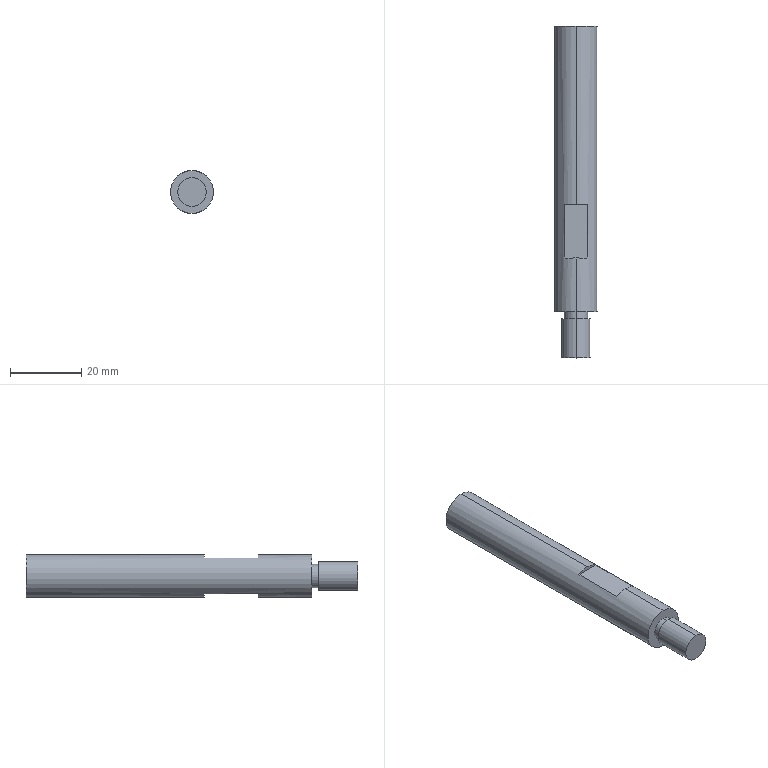Part | STEP file | PN_0059 pillar | 1 solid | 20 faces | box 12 x 93 x 12 mm | volume 9356 mm3 | plane 10 | cylinder 8 | cone 2 | commonest cylinder face diameters 4.2 x2 6.6 x2 8 x2 12 x2
STEP:
#1=CARTESIAN_POINT('',(0.,0.,0.));
#2=DIRECTION('',(0.,0.,1.));
#3=DIRECTION('',(1.,0.,0.));
#4=AXIS2_PLACEMENT_3D('',#1,#2,#3);
#5=CARTESIAN_POINT('',(0.,11.,-4.));
#6=VERTEX_POINT('',#5);
#7=CARTESIAN_POINT('',(0.,11.,4.));
#8=VERTEX_POINT('',#7);
#9=CARTESIAN_POINT('',(0.,11.,0.));
#10=DIRECTION('',(0.,-1.,0.));
#11=DIRECTION('',(0.,0.,-1.));
#12=AXIS2_PLACEMENT_3D('',#9,#10,#11);
#13=CIRCLE('',#12,4.);
#14=CARTESIAN_POINT('',(0.,0.,0.));
#15=DIRECTION('',(0.,-1.,0.));
#16=DIRECTION('',(0.,0.,-1.));
#17=AXIS2_PLACEMENT_3D('',#14,#15,#16);
#18=CYLINDRICAL_SURFACE('',#17,4.);
#19=CARTESIAN_POINT('',(0.,-11.));
#20=DIRECTION('',(1.,0.));
#21=VECTOR('',#20,1.);
#22=LINE('',#19,#21);
#23=(GEOMETRIC_REPRESENTATION_CONTEXT(2)PARAMETRIC_REPRESENTATION_CONTEXT()REPRESENTATION_CONTEXT('',''));
#24=DEFINITIONAL_REPRESENTATION('',(#22),#23);
#25=PCURVE('',#18,#24);
#26=CARTESIAN_POINT('',(4.,11.,0.));
#27=DIRECTION('',(0.,-1.,0.));
#28=DIRECTION('',(0.,0.,-1.));
#29=AXIS2_PLACEMENT_3D('',#26,#27,#28);
#30=PLANE('',#29);
#31=CARTESIAN_POINT('',(0.,-4.));
#32=DIRECTION('',(1.,0.));
#33=AXIS2_PLACEMENT_2D('',#31,#32);
#34=CIRCLE('',#33,4.);
#35=(GEOMETRIC_REPRESENTATION_CONTEXT(2)PARAMETRIC_REPRESENTATION_CONTEXT()REPRESENTATION_CONTEXT('',''));
#36=DEFINITIONAL_REPRESENTATION('',(#34),#35);
#37=PCURVE('',#30,#36);
#38=SURFACE_CURVE('',#13,(#25,#37),.PCURVE_S1.);
#39=EDGE_CURVE('',#6,#8,#38,.T.);
#40=ORIENTED_EDGE('',*,*,#39,.T.);
#41=CARTESIAN_POINT('',(0.,0.,4.));
#42=VERTEX_POINT('',#41);
#43=CARTESIAN_POINT('',(0.,0.,4.));
#44=DIRECTION('',(0.,-1.,0.));
#45=VECTOR('',#44,1.);
#46=LINE('',#43,#45);
#47=CARTESIAN_POINT('',(3.142,0.));
#48=DIRECTION('',(0.,1.));
#49=VECTOR('',#48,1.);
#50=LINE('',#47,#49);
#51=(GEOMETRIC_REPRESENTATION_CONTEXT(2)PARAMETRIC_REPRESENTATION_CONTEXT()REPRESENTATION_CONTEXT('',''));
#52=DEFINITIONAL_REPRESENTATION('',(#50),#51);
#53=PCURVE('',#18,#52);
#54=CARTESIAN_POINT('',(0.,0.,0.));
#55=DIRECTION('',(0.,-1.,0.));
#56=DIRECTION('',(0.,0.,-1.));
#57=AXIS2_PLACEMENT_3D('',#54,#55,#56);
#58=CYLINDRICAL_SURFACE('',#57,4.);
#59=CARTESIAN_POINT('',(3.142,0.));
#60=DIRECTION('',(0.,1.));
#61=VECTOR('',#60,1.);
#62=LINE('',#59,#61);
#63=(GEOMETRIC_REPRESENTATION_CONTEXT(2)PARAMETRIC_REPRESENTATION_CONTEXT()REPRESENTATION_CONTEXT('',''));
#64=DEFINITIONAL_REPRESENTATION('',(#62),#63);
#65=PCURVE('',#58,#64);
#66=SURFACE_CURVE('',#46,(#53,#65),.PCURVE_S1.);
#67=EDGE_CURVE('',#8,#42,#66,.T.);
#68=ORIENTED_EDGE('',*,*,#67,.T.);
#69=CARTESIAN_POINT('',(0.,0.,-4.));
#70=VERTEX_POINT('',#69);
#71=CARTESIAN_POINT('',(0.,0.,0.));
#72=DIRECTION('',(0.,-1.,0.));
#73=DIRECTION('',(0.,0.,-1.));
#74=AXIS2_PLACEMENT_3D('',#71,#72,#73);
#75=CIRCLE('',#74,4.);
#76=CARTESIAN_POINT('',(0.,0.));
#77=DIRECTION('',(1.,0.));
#78=VECTOR('',#77,1.);
#79=LINE('',#76,#78);
#80=(GEOMETRIC_REPRESENTATION_CONTEXT(2)PARAMETRIC_REPRESENTATION_CONTEXT()REPRESENTATION_CONTEXT('',''));
#81=DEFINITIONAL_REPRESENTATION('',(#79),#80);
#82=PCURVE('',#18,#81);
#83=CARTESIAN_POINT('',(0.,0.,0.));
#84=DIRECTION('',(0.,-1.,0.));
#85=DIRECTION('',(0.,0.,-1.));
#86=AXIS2_PLACEMENT_3D('',#83,#84,#85);
#87=PLANE('',#86);
#88=CARTESIAN_POINT('',(0.,0.));
#89=DIRECTION('',(1.,0.));
#90=AXIS2_PLACEMENT_2D('',#88,#89);
#91=CIRCLE('',#90,4.);
#92=(GEOMETRIC_REPRESENTATION_CONTEXT(2)PARAMETRIC_REPRESENTATION_CONTEXT()REPRESENTATION_CONTEXT('',''));
#93=DEFINITIONAL_REPRESENTATION('',(#91),#92);
#94=PCURVE('',#87,#93);
#95=SURFACE_CURVE('',#75,(#82,#94),.PCURVE_S1.);
#96=EDGE_CURVE('',#70,#42,#95,.T.);
#97=ORIENTED_EDGE('',*,*,#96,.F.);
#98=CARTESIAN_POINT('',(0.,0.,-4.));
#99=DIRECTION('',(0.,-1.,0.));
#100=VECTOR('',#99,1.);
#101=LINE('',#98,#100);
#102=CARTESIAN_POINT('',(0.,0.));
#103=DIRECTION('',(0.,1.));
#104=VECTOR('',#103,1.);
#105=LINE('',#102,#104);
#106=(GEOMETRIC_REPRESENTATION_CONTEXT(2)PARAMETRIC_REPRESENTATION_CONTEXT()REPRESENTATION_CONTEXT('',''));
#107=DEFINITIONAL_REPRESENTATION('',(#105),#106);
#108=PCURVE('',#18,#107);
#109=CARTESIAN_POINT('',(6.283,0.));
#110=DIRECTION('',(0.,1.));
#111=VECTOR('',#110,1.);
#112=LINE('',#109,#111);
#113=(GEOMETRIC_REPRESENTATION_CONTEXT(2)PARAMETRIC_REPRESENTATION_CONTEXT()REPRESENTATION_CONTEXT('',''));
#114=DEFINITIONAL_REPRESENTATION('',(#112),#113);
#115=PCURVE('',#58,#114);
#116=SURFACE_CURVE('',#101,(#108,#115),.PCURVE_S1.);
#117=EDGE_CURVE('',#6,#70,#116,.T.);
#118=ORIENTED_EDGE('',*,*,#117,.F.);
#119=EDGE_LOOP('',(#40,#68,#97,#118));
#120=FACE_BOUND('',#119,.T.);
#121=ADVANCED_FACE('',(#120),#18,.T.);
#122=CARTESIAN_POINT('',(0.,13.,-3.3));
#123=VERTEX_POINT('',#122);
#124=CARTESIAN_POINT('',(0.,13.,3.3));
#125=VERTEX_POINT('',#124);
#126=CARTESIAN_POINT('',(0.,13.,0.));
#127=DIRECTION('',(0.,-1.,0.));
#128=DIRECTION('',(0.,0.,-1.));
#129=AXIS2_PLACEMENT_3D('',#126,#127,#128);
#130=CIRCLE('',#129,3.3);
#131=CARTESIAN_POINT('',(0.,0.,0.));
#132=DIRECTION('',(0.,-1.,0.));
#133=DIRECTION('',(0.,0.,-1.));
#134=AXIS2_PLACEMENT_3D('',#131,#132,#133);
#135=CYLINDRICAL_SURFACE('',#134,3.3);
#136=CARTESIAN_POINT('',(0.,-13.));
#137=DIRECTION('',(1.,0.));
#138=VECTOR('',#137,1.);
#139=LINE('',#136,#138);
#140=(GEOMETRIC_REPRESENTATION_CONTEXT(2)PARAMETRIC_REPRESENTATION_CONTEXT()REPRESENTATION_CONTEXT('',''));
#141=DEFINITIONAL_REPRESENTATION('',(#139),#140);
#142=PCURVE('',#135,#141);
#143=CARTESIAN_POINT('',(4.,13.,0.));
#144=DIRECTION('',(0.,-1.,0.));
#145=DIRECTION('',(0.,0.,-1.));
#146=AXIS2_PLACEMENT_3D('',#143,#144,#145);
#147=PLANE('',#146);
#148=CARTESIAN_POINT('',(0.,-4.));
#149=DIRECTION('',(1.,0.));
#150=AXIS2_PLACEMENT_2D('',#148,#149);
#151=CIRCLE('',#150,3.3);
#152=(GEOMETRIC_REPRESENTATION_CONTEXT(2)PARAMETRIC_REPRESENTATION_CONTEXT()REPRESENTATION_CONTEXT('',''));
#153=DEFINITIONAL_REPRESENTATION('',(#151),#152);
#154=PCURVE('',#147,#153);
#155=SURFACE_CURVE('',#130,(#142,#154),.PCURVE_S1.);
#156=EDGE_CURVE('',#123,#125,#155,.T.);
#157=ORIENTED_EDGE('',*,*,#156,.T.);
#158=CARTESIAN_POINT('',(0.,11.,3.3));
#159=VERTEX_POINT('',#158);
#160=CARTESIAN_POINT('',(0.,0.,3.3));
#161=DIRECTION('',(0.,-1.,0.));
#162=VECTOR('',#161,1.);
#163=LINE('',#160,#162);
#164=CARTESIAN_POINT('',(3.142,0.));
#165=DIRECTION('',(0.,1.));
#166=VECTOR('',#165,1.);
#167=LINE('',#164,#166);
#168=(GEOMETRIC_REPRESENTATION_CONTEXT(2)PARAMETRIC_REPRESENTATION_CONTEXT()REPRESENTATION_CONTEXT('',''));
#169=DEFINITIONAL_REPRESENTATION('',(#167),#168);
#170=PCURVE('',#135,#169);
#171=CARTESIAN_POINT('',(0.,0.,0.));
#172=DIRECTION('',(0.,-1.,0.));
#173=DIRECTION('',(0.,0.,-1.));
#174=AXIS2_PLACEMENT_3D('',#171,#172,#173);
#175=CYLINDRICAL_SURFACE('',#174,3.3);
#176=CARTESIAN_POINT('',(3.142,0.));
#177=DIRECTION('',(0.,1.));
#178=VECTOR('',#177,1.);
#179=LINE('',#176,#178);
#180=(GEOMETRIC_REPRESENTATION_CONTEXT(2)PARAMETRIC_REPRESENTATION_CONTEXT()REPRESENTATION_CONTEXT('',''));
#181=DEFINITIONAL_REPRESENTATION('',(#179),#180);
#182=PCURVE('',#175,#181);
#183=SURFACE_CURVE('',#163,(#170,#182),.PCURVE_S1.);
#184=EDGE_CURVE('',#125,#159,#183,.T.);
#185=ORIENTED_EDGE('',*,*,#184,.T.);
#186=CARTESIAN_POINT('',(0.,11.,-3.3));
#187=VERTEX_POINT('',#186);
#188=CARTESIAN_POINT('',(0.,11.,0.));
#189=DIRECTION('',(0.,-1.,0.));
#190=DIRECTION('',(0.,0.,-1.));
#191=AXIS2_PLACEMENT_3D('',#188,#189,#190);
#192=CIRCLE('',#191,3.3);
#193=CARTESIAN_POINT('',(0.,-11.));
#194=DIRECTION('',(1.,0.));
#195=VECTOR('',#194,1.);
#196=LINE('',#193,#195);
#197=(GEOMETRIC_REPRESENTATION_CONTEXT(2)PARAMETRIC_REPRESENTATION_CONTEXT()REPRESENTATION_CONTEXT('',''));
#198=DEFINITIONAL_REPRESENTATION('',(#196),#197);
#199=PCURVE('',#135,#198);
#200=CARTESIAN_POINT('',(0.,-4.));
#201=DIRECTION('',(1.,0.));
#202=AXIS2_PLACEMENT_2D('',#200,#201);
#203=CIRCLE('',#202,3.3);
#204=(GEOMETRIC_REPRESENTATION_CONTEXT(2)PARAMETRIC_REPRESENTATION_CONTEXT()REPRESENTATION_CONTEXT('',''));
#205=DEFINITIONAL_REPRESENTATION('',(#203),#204);
#206=PCURVE('',#30,#205);
#207=SURFACE_CURVE('',#192,(#199,#206),.PCURVE_S1.);
#208=EDGE_CURVE('',#187,#159,#207,.T.);
#209=ORIENTED_EDGE('',*,*,#208,.F.);
#210=CARTESIAN_POINT('',(0.,0.,-3.3));
#211=DIRECTION('',(0.,-1.,0.));
#212=VECTOR('',#211,1.);
#213=LINE('',#210,#212);
#214=CARTESIAN_POINT('',(0.,0.));
#215=DIRECTION('',(0.,1.));
#216=VECTOR('',#215,1.);
#217=LINE('',#214,#216);
#218=(GEOMETRIC_REPRESENTATION_CONTEXT(2)PARAMETRIC_REPRESENTATION_CONTEXT()REPRESENTATION_CONTEXT('',''));
#219=DEFINITIONAL_REPRESENTATION('',(#217),#218);
#220=PCURVE('',#135,#219);
#221=CARTESIAN_POINT('',(6.283,0.));
#222=DIRECTION('',(0.,1.));
#223=VECTOR('',#222,1.);
#224=LINE('',#221,#223);
#225=(GEOMETRIC_REPRESENTATION_CONTEXT(2)PARAMETRIC_REPRESENTATION_CONTEXT()REPRESENTATION_CONTEXT('',''));
#226=DEFINITIONAL_REPRESENTATION('',(#224),#225);
#227=PCURVE('',#175,#226);
#228=SURFACE_CURVE('',#213,(#220,#227),.PCURVE_S1.);
#229=EDGE_CURVE('',#123,#187,#228,.T.);
#230=ORIENTED_EDGE('',*,*,#229,.F.);
#231=EDGE_LOOP('',(#157,#185,#209,#230));
#232=FACE_BOUND('',#231,.T.);
#233=ADVANCED_FACE('',(#232),#135,.T.);
#234=CARTESIAN_POINT('',(0.,80.6,2.1));
#235=VERTEX_POINT('',#234);
#236=CARTESIAN_POINT('',(0.,93.,2.1));
#237=VERTEX_POINT('',#236);
#238=CARTESIAN_POINT('',(0.,93.,2.1));
#239=DIRECTION('',(0.,1.,0.));
#240=VECTOR('',#239,1.);
#241=LINE('',#238,#240);
#242=CARTESIAN_POINT('',(0.,93.,0.));
#243=DIRECTION('',(0.,1.,0.));
#244=DIRECTION('',(0.,0.,1.));
#245=AXIS2_PLACEMENT_3D('',#242,#243,#244);
#246=CYLINDRICAL_SURFACE('',#245,2.1);
#247=CARTESIAN_POINT('',(6.283,0.));
#248=DIRECTION('',(0.,1.));
#249=VECTOR('',#248,1.);
#250=LINE('',#247,#249);
#251=(GEOMETRIC_REPRESENTATION_CONTEXT(2)PARAMETRIC_REPRESENTATION_CONTEXT()REPRESENTATION_CONTEXT('',''));
#252=DEFINITIONAL_REPRESENTATION('',(#250),#251);
#253=PCURVE('',#246,#252);
#254=CARTESIAN_POINT('',(0.,93.,0.));
#255=DIRECTION('',(0.,1.,0.));
#256=DIRECTION('',(0.,0.,1.));
#257=AXIS2_PLACEMENT_3D('',#254,#255,#256);
#258=CYLINDRICAL_SURFACE('',#257,2.1);
#259=CARTESIAN_POINT('',(0.,0.));
#260=DIRECTION('',(0.,1.));
#261=VECTOR('',#260,1.);
#262=LINE('',#259,#261);
#263=(GEOMETRIC_REPRESENTATION_CONTEXT(2)PARAMETRIC_REPRESENTATION_CONTEXT()REPRESENTATION_CONTEXT('',''));
#264=DEFINITIONAL_REPRESENTATION('',(#262),#263);
#265=PCURVE('',#258,#264);
#266=SURFACE_CURVE('',#241,(#253,#265),.PCURVE_S1.);
#267=EDGE_CURVE('',#235,#237,#266,.T.);
#268=ORIENTED_EDGE('',*,*,#267,.T.);
#269=CARTESIAN_POINT('',(0.,93.,-2.1));
#270=VERTEX_POINT('',#269);
#271=CARTESIAN_POINT('',(0.,93.,0.));
#272=DIRECTION('',(0.,1.,0.));
#273=DIRECTION('',(0.,0.,1.));
#274=AXIS2_PLACEMENT_3D('',#271,#272,#273);
#275=CIRCLE('',#274,2.1);
#276=CARTESIAN_POINT('',(0.,0.));
#277=DIRECTION('',(1.,0.));
#278=VECTOR('',#277,1.);
#279=LINE('',#276,#278);
#280=(GEOMETRIC_REPRESENTATION_CONTEXT(2)PARAMETRIC_REPRESENTATION_CONTEXT()REPRESENTATION_CONTEXT('',''));
#281=DEFINITIONAL_REPRESENTATION('',(#279),#280);
#282=PCURVE('',#246,#281);
#283=CARTESIAN_POINT('',(6.,93.,0.));
#284=DIRECTION('',(0.,1.,0.));
#285=DIRECTION('',(0.,0.,1.));
#286=AXIS2_PLACEMENT_3D('',#283,#284,#285);
#287=PLANE('',#286);
#288=CARTESIAN_POINT('',(0.,-6.));
#289=DIRECTION('',(1.,0.));
#290=AXIS2_PLACEMENT_2D('',#288,#289);
#291=CIRCLE('',#290,2.1);
#292=(GEOMETRIC_REPRESENTATION_CONTEXT(2)PARAMETRIC_REPRESENTATION_CONTEXT()REPRESENTATION_CONTEXT('',''));
#293=DEFINITIONAL_REPRESENTATION('',(#291),#292);
#294=PCURVE('',#287,#293);
#295=SURFACE_CURVE('',#275,(#282,#294),.PCURVE_S1.);
#296=EDGE_CURVE('',#270,#237,#295,.T.);
#297=ORIENTED_EDGE('',*,*,#296,.F.);
#298=CARTESIAN_POINT('',(0.,80.6,-2.1));
#299=VERTEX_POINT('',#298);
#300=CARTESIAN_POINT('',(0.,93.,-2.1));
#301=DIRECTION('',(0.,1.,0.));
#302=VECTOR('',#301,1.);
#303=LINE('',#300,#302);
#304=CARTESIAN_POINT('',(3.142,0.));
#305=DIRECTION('',(0.,1.));
#306=VECTOR('',#305,1.);
#307=LINE('',#304,#306);
#308=(GEOMETRIC_REPRESENTATION_CONTEXT(2)PARAMETRIC_REPRESENTATION_CONTEXT()REPRESENTATION_CONTEXT('',''));
#309=DEFINITIONAL_REPRESENTATION('',(#307),#308);
#310=PCURVE('',#246,#309);
#311=CARTESIAN_POINT('',(3.142,0.));
#312=DIRECTION('',(0.,1.));
#313=VECTOR('',#312,1.);
#314=LINE('',#311,#313);
#315=(GEOMETRIC_REPRESENTATION_CONTEXT(2)PARAMETRIC_REPRESENTATION_CONTEXT()REPRESENTATION_CONTEXT('',''));
#316=DEFINITIONAL_REPRESENTATION('',(#314),#315);
#317=PCURVE('',#258,#316);
#318=SURFACE_CURVE('',#303,(#310,#317),.PCURVE_S1.);
#319=EDGE_CURVE('',#299,#270,#318,.T.);
#320=ORIENTED_EDGE('',*,*,#319,.F.);
#321=CARTESIAN_POINT('',(0.,80.6,0.));
#322=DIRECTION('',(0.,1.,0.));
#323=DIRECTION('',(0.,0.,1.));
#324=AXIS2_PLACEMENT_3D('',#321,#322,#323);
#325=CIRCLE('',#324,2.1);
#326=CARTESIAN_POINT('',(0.,-12.4));
#327=DIRECTION('',(1.,0.));
#328=VECTOR('',#327,1.);
#329=LINE('',#326,#328);
#330=(GEOMETRIC_REPRESENTATION_CONTEXT(2)PARAMETRIC_REPRESENTATION_CONTEXT()REPRESENTATION_CONTEXT('',''));
#331=DEFINITIONAL_REPRESENTATION('',(#329),#330);
#332=PCURVE('',#246,#331);
#333=CARTESIAN_POINT('',(0.,80.6,0.));
#334=DIRECTION('',(0.,1.,0.));
#335=DIRECTION('',(0.,0.,1.));
#336=AXIS2_PLACEMENT_3D('',#333,#334,#335);
#337=CONICAL_SURFACE('',#336,2.1,1.03);
#338=CARTESIAN_POINT('',(0.,0.));
#339=DIRECTION('',(1.,0.));
#340=VECTOR('',#339,1.);
#341=LINE('',#338,#340);
#342=(GEOMETRIC_REPRESENTATION_CONTEXT(2)PARAMETRIC_REPRESENTATION_CONTEXT()REPRESENTATION_CONTEXT('',''));
#343=DEFINITIONAL_REPRESENTATION('',(#341),#342);
#344=PCURVE('',#337,#343);
#345=SURFACE_CURVE('',#325,(#332,#344),.PCURVE_S1.);
#346=EDGE_CURVE('',#299,#235,#345,.T.);
#347=ORIENTED_EDGE('',*,*,#346,.T.);
#348=EDGE_LOOP('',(#268,#297,#320,#347));
#349=FACE_BOUND('',#348,.F.);
#350=ADVANCED_FACE('',(#349),#246,.F.);
#351=ORIENTED_EDGE('',*,*,#346,.F.);
#352=CARTESIAN_POINT('',(0.,79.338,0.));
#353=VERTEX_POINT('',#352);
#354=CARTESIAN_POINT('',(0.,80.6,-2.1));
#355=DIRECTION('',(0.,0.515,-0.8572));
#356=VECTOR('',#355,1.);
#357=LINE('',#354,#356);
#358=CARTESIAN_POINT('',(3.142,0.));
#359=DIRECTION('',(0.,1.));
#360=VECTOR('',#359,1.);
#361=LINE('',#358,#360);
#362=(GEOMETRIC_REPRESENTATION_CONTEXT(2)PARAMETRIC_REPRESENTATION_CONTEXT()REPRESENTATION_CONTEXT('',''));
#363=DEFINITIONAL_REPRESENTATION('',(#361),#362);
#364=PCURVE('',#337,#363);
#365=CARTESIAN_POINT('',(0.,80.6,0.));
#366=DIRECTION('',(0.,1.,0.));
#367=DIRECTION('',(0.,0.,1.));
#368=AXIS2_PLACEMENT_3D('',#365,#366,#367);
#369=CONICAL_SURFACE('',#368,2.1,1.03);
#370=CARTESIAN_POINT('',(3.142,0.));
#371=DIRECTION('',(0.,1.));
#372=VECTOR('',#371,1.);
#373=LINE('',#370,#372);
#374=(GEOMETRIC_REPRESENTATION_CONTEXT(2)PARAMETRIC_REPRESENTATION_CONTEXT()REPRESENTATION_CONTEXT('',''));
#375=DEFINITIONAL_REPRESENTATION('',(#373),#374);
#376=PCURVE('',#369,#375);
#377=SURFACE_CURVE('',#357,(#364,#376),.PCURVE_S1.);
#378=EDGE_CURVE('',#353,#299,#377,.T.);
#379=ORIENTED_EDGE('',*,*,#378,.F.);
#380=CARTESIAN_POINT('',(0.,80.6,2.1));
#381=DIRECTION('',(0.,0.515,0.8572));
#382=VECTOR('',#381,1.);
#383=LINE('',#380,#382);
#384=CARTESIAN_POINT('',(6.283,0.));
#385=DIRECTION('',(0.,1.));
#386=VECTOR('',#385,1.);
#387=LINE('',#384,#386);
#388=(GEOMETRIC_REPRESENTATION_CONTEXT(2)PARAMETRIC_REPRESENTATION_CONTEXT()REPRESENTATION_CONTEXT('',''));
#389=DEFINITIONAL_REPRESENTATION('',(#387),#388);
#390=PCURVE('',#337,#389);
#391=CARTESIAN_POINT('',(0.,0.));
#392=DIRECTION('',(0.,1.));
#393=VECTOR('',#392,1.);
#394=LINE('',#391,#393);
#395=(GEOMETRIC_REPRESENTATION_CONTEXT(2)PARAMETRIC_REPRESENTATION_CONTEXT()REPRESENTATION_CONTEXT('',''));
#396=DEFINITIONAL_REPRESENTATION('',(#394),#395);
#397=PCURVE('',#369,#396);
#398=SURFACE_CURVE('',#383,(#390,#397),.PCURVE_S1.);
#399=EDGE_CURVE('',#353,#235,#398,.T.);
#400=ORIENTED_EDGE('',*,*,#399,.T.);
#401=EDGE_LOOP('',(#351,#379,#400));
#402=FACE_BOUND('',#401,.F.);
#403=ADVANCED_FACE('',(#402),#337,.F.);
#404=CARTESIAN_POINT('',(0.,93.,-6.));
#405=VERTEX_POINT('',#404);
#406=CARTESIAN_POINT('',(0.,93.,6.));
#407=VERTEX_POINT('',#406);
#408=CARTESIAN_POINT('',(0.,93.,0.));
#409=DIRECTION('',(0.,-1.,0.));
#410=DIRECTION('',(0.,0.,-1.));
#411=AXIS2_PLACEMENT_3D('',#408,#409,#410);
#412=CIRCLE('',#411,6.);
#413=CARTESIAN_POINT('',(0.,0.,0.));
#414=DIRECTION('',(0.,-1.,0.));
#415=DIRECTION('',(0.,0.,-1.));
#416=AXIS2_PLACEMENT_3D('',#413,#414,#415);
#417=CYLINDRICAL_SURFACE('',#416,6.);
#418=CARTESIAN_POINT('',(0.,-93.));
#419=DIRECTION('',(1.,0.));
#420=VECTOR('',#419,1.);
#421=LINE('',#418,#420);
#422=(GEOMETRIC_REPRESENTATION_CONTEXT(2)PARAMETRIC_REPRESENTATION_CONTEXT()REPRESENTATION_CONTEXT('',''));
#423=DEFINITIONAL_REPRESENTATION('',(#421),#422);
#424=PCURVE('',#417,#423);
#425=CARTESIAN_POINT('',(-6.,-6.));
#426=CARTESIAN_POINT('',(-6.,4.392));
#427=CARTESIAN_POINT('',(3.,-0.8038));
#428=CARTESIAN_POINT('',(12.,-6.));
#429=CARTESIAN_POINT('',(3.,-11.196));
#430=CARTESIAN_POINT('',(-6.,-16.392));
#431=CARTESIAN_POINT('',(-6.,-6.));
#432=(BOUNDED_CURVE()B_SPLINE_CURVE(2,(#425,#426,#427,#428,#429,#430,#431),.UNSPECIFIED.,.T.,.F.)B_SPLINE_CURVE_WITH_KNOTS((1,2,2,2,2,1),(-2.094,0.,2.094,4.189,6.283,8.378),.UNSPECIFIED.)CURVE()GEOMETRIC_REPRESENTATION_ITEM()RATIONAL_B_SPLINE_CURVE((1.,0.5,1.,0.5,1.,0.5,1.))REPRESENTATION_ITEM(''));
#433=(GEOMETRIC_REPRESENTATION_CONTEXT(2)PARAMETRIC_REPRESENTATION_CONTEXT()REPRESENTATION_CONTEXT('',''));
#434=DEFINITIONAL_REPRESENTATION('',(#432),#433);
#435=PCURVE('',#287,#434);
#436=SURFACE_CURVE('',#412,(#424,#435),.PCURVE_S1.);
#437=EDGE_CURVE('',#405,#407,#436,.T.);
#438=ORIENTED_EDGE('',*,*,#437,.T.);
#439=CARTESIAN_POINT('',(0.,43.,6.));
#440=VERTEX_POINT('',#439);
#441=CARTESIAN_POINT('',(0.,0.,6.));
#442=DIRECTION('',(0.,-1.,0.));
#443=VECTOR('',#442,1.);
#444=LINE('',#441,#443);
#445=CARTESIAN_POINT('',(3.142,0.));
#446=DIRECTION('',(0.,1.));
#447=VECTOR('',#446,1.);
#448=LINE('',#445,#447);
#449=(GEOMETRIC_REPRESENTATION_CONTEXT(2)PARAMETRIC_REPRESENTATION_CONTEXT()REPRESENTATION_CONTEXT('',''));
#450=DEFINITIONAL_REPRESENTATION('',(#448),#449);
#451=PCURVE('',#417,#450);
#452=CARTESIAN_POINT('',(0.,0.,0.));
#453=DIRECTION('',(0.,-1.,0.));
#454=DIRECTION('',(0.,0.,-1.));
#455=AXIS2_PLACEMENT_3D('',#452,#453,#454);
#456=CYLINDRICAL_SURFACE('',#455,6.);
#457=CARTESIAN_POINT('',(3.142,0.));
#458=DIRECTION('',(0.,1.));
#459=VECTOR('',#458,1.);
#460=LINE('',#457,#459);
#461=(GEOMETRIC_REPRESENTATION_CONTEXT(2)PARAMETRIC_REPRESENTATION_CONTEXT()REPRESENTATION_CONTEXT('',''));
#462=DEFINITIONAL_REPRESENTATION('',(#460),#461);
#463=PCURVE('',#456,#462);
#464=SURFACE_CURVE('',#444,(#451,#463),.PCURVE_S1.);
#465=EDGE_CURVE('',#407,#440,#464,.T.);
#466=ORIENTED_EDGE('',*,*,#465,.T.);
#467=CARTESIAN_POINT('',(3.317,43.,5.));
#468=VERTEX_POINT('',#467);
#469=CARTESIAN_POINT('',(0.,43.,0.));
#470=DIRECTION('',(0.,-1.,0.));
#471=DIRECTION('',(0.,0.,1.));
#472=AXIS2_PLACEMENT_3D('',#469,#470,#471);
#473=CIRCLE('',#472,6.);
#474=CARTESIAN_POINT('',(-3.142,-43.));
#475=DIRECTION('',(1.,0.));
#476=VECTOR('',#475,1.);
#477=LINE('',#474,#476);
#478=(GEOMETRIC_REPRESENTATION_CONTEXT(2)PARAMETRIC_REPRESENTATION_CONTEXT()REPRESENTATION_CONTEXT('',''));
#479=DEFINITIONAL_REPRESENTATION('',(#477),#478);
#480=PCURVE('',#417,#479);
#481=CARTESIAN_POINT('',(-35.,43.,8.217));
#482=DIRECTION('',(0.,1.,0.));
#483=DIRECTION('',(0.,0.,1.));
#484=AXIS2_PLACEMENT_3D('',#481,#482,#483);
#485=PLANE('',#484);
#486=CARTESIAN_POINT('',(-2.217,35.));
#487=CARTESIAN_POINT('',(-2.217,24.608));
#488=CARTESIAN_POINT('',(-11.217,29.804));
#489=CARTESIAN_POINT('',(-20.217,35.));
#490=CARTESIAN_POINT('',(-11.217,40.196));
#491=CARTESIAN_POINT('',(-2.217,45.392));
#492=CARTESIAN_POINT('',(-2.217,35.));
#493=(BOUNDED_CURVE()B_SPLINE_CURVE(2,(#486,#487,#488,#489,#490,#491,#492),.UNSPECIFIED.,.T.,.F.)B_SPLINE_CURVE_WITH_KNOTS((1,2,2,2,2,1),(-2.094,0.,2.094,4.189,6.283,8.378),.UNSPECIFIED.)CURVE()GEOMETRIC_REPRESENTATION_ITEM()RATIONAL_B_SPLINE_CURVE((1.,0.5,1.,0.5,1.,0.5,1.))REPRESENTATION_ITEM(''));
#494=(GEOMETRIC_REPRESENTATION_CONTEXT(2)PARAMETRIC_REPRESENTATION_CONTEXT()REPRESENTATION_CONTEXT('',''));
#495=DEFINITIONAL_REPRESENTATION('',(#493),#494);
#496=PCURVE('',#485,#495);
#497=SURFACE_CURVE('',#473,(#480,#496),.PCURVE_S1.);
#498=EDGE_CURVE('',#468,#440,#497,.T.);
#499=ORIENTED_EDGE('',*,*,#498,.F.);
#500=CARTESIAN_POINT('',(3.317,28.,5.));
#501=VERTEX_POINT('',#500);
#502=CARTESIAN_POINT('',(3.317,0.,5.));
#503=DIRECTION('',(0.,1.,0.));
#504=VECTOR('',#503,1.);
#505=LINE('',#502,#504);
#506=CARTESIAN_POINT('',(2.556,0.));
#507=DIRECTION('',(0.,-1.));
#508=VECTOR('',#507,1.);
#509=LINE('',#506,#508);
#510=(GEOMETRIC_REPRESENTATION_CONTEXT(2)PARAMETRIC_REPRESENTATION_CONTEXT()REPRESENTATION_CONTEXT('',''));
#511=DEFINITIONAL_REPRESENTATION('',(#509),#510);
#512=PCURVE('',#417,#511);
#513=CARTESIAN_POINT('',(-35.,43.,5.));
#514=DIRECTION('',(0.,0.,-1.));
#515=DIRECTION('',(0.,1.,0.));
#516=AXIS2_PLACEMENT_3D('',#513,#514,#515);
#517=PLANE('',#516);
#518=CARTESIAN_POINT('',(-43.,38.317));
#519=DIRECTION('',(1.,0.));
#520=VECTOR('',#519,1.);
#521=LINE('',#518,#520);
#522=(GEOMETRIC_REPRESENTATION_CONTEXT(2)PARAMETRIC_REPRESENTATION_CONTEXT()REPRESENTATION_CONTEXT('',''));
#523=DEFINITIONAL_REPRESENTATION('',(#521),#522);
#524=PCURVE('',#517,#523);
#525=SURFACE_CURVE('',#505,(#512,#524),.PCURVE_S1.);
#526=EDGE_CURVE('',#501,#468,#525,.T.);
#527=ORIENTED_EDGE('',*,*,#526,.F.);
#528=CARTESIAN_POINT('',(0.,28.,6.));
#529=VERTEX_POINT('',#528);
#530=CARTESIAN_POINT('',(0.,28.,0.));
#531=DIRECTION('',(0.,1.,0.));
#532=DIRECTION('',(0.,0.,-1.));
#533=AXIS2_PLACEMENT_3D('',#530,#531,#532);
#534=CIRCLE('',#533,6.);
#535=CARTESIAN_POINT('',(6.283,-28.));
#536=DIRECTION('',(-1.,0.));
#537=VECTOR('',#536,1.);
#538=LINE('',#535,#537);
#539=(GEOMETRIC_REPRESENTATION_CONTEXT(2)PARAMETRIC_REPRESENTATION_CONTEXT()REPRESENTATION_CONTEXT('',''));
#540=DEFINITIONAL_REPRESENTATION('',(#538),#539);
#541=PCURVE('',#417,#540);
#542=CARTESIAN_POINT('',(-35.,28.,8.217));
#543=DIRECTION('',(0.,-1.,0.));
#544=DIRECTION('',(0.,0.,-1.));
#545=AXIS2_PLACEMENT_3D('',#542,#543,#544);
#546=PLANE('',#545);
#547=CARTESIAN_POINT('',(14.217,35.));
#548=CARTESIAN_POINT('',(14.217,24.608));
#549=CARTESIAN_POINT('',(5.217,29.804));
#550=CARTESIAN_POINT('',(-3.783,35.));
#551=CARTESIAN_POINT('',(5.217,40.196));
#552=CARTESIAN_POINT('',(14.217,45.392));
#553=CARTESIAN_POINT('',(14.217,35.));
#554=(BOUNDED_CURVE()B_SPLINE_CURVE(2,(#547,#548,#549,#550,#551,#552,#553),.UNSPECIFIED.,.T.,.F.)B_SPLINE_CURVE_WITH_KNOTS((1,2,2,2,2,1),(-2.094,0.,2.094,4.189,6.283,8.378),.UNSPECIFIED.)CURVE()GEOMETRIC_REPRESENTATION_ITEM()RATIONAL_B_SPLINE_CURVE((1.,0.5,1.,0.5,1.,0.5,1.))REPRESENTATION_ITEM(''));
#555=(GEOMETRIC_REPRESENTATION_CONTEXT(2)PARAMETRIC_REPRESENTATION_CONTEXT()REPRESENTATION_CONTEXT('',''));
#556=DEFINITIONAL_REPRESENTATION('',(#554),#555);
#557=PCURVE('',#546,#556);
#558=SURFACE_CURVE('',#534,(#541,#557),.PCURVE_S1.);
#559=EDGE_CURVE('',#529,#501,#558,.T.);
#560=ORIENTED_EDGE('',*,*,#559,.F.);
#561=CARTESIAN_POINT('',(0.,13.,6.));
#562=VERTEX_POINT('',#561);
#563=CARTESIAN_POINT('',(0.,0.,6.));
#564=DIRECTION('',(0.,-1.,0.));
#565=VECTOR('',#564,1.);
#566=LINE('',#563,#565);
#567=CARTESIAN_POINT('',(3.142,0.));
#568=DIRECTION('',(0.,1.));
#569=VECTOR('',#568,1.);
#570=LINE('',#567,#569);
#571=(GEOMETRIC_REPRESENTATION_CONTEXT(2)PARAMETRIC_REPRESENTATION_CONTEXT()REPRESENTATION_CONTEXT('',''));
#572=DEFINITIONAL_REPRESENTATION('',(#570),#571);
#573=PCURVE('',#417,#572);
#574=CARTESIAN_POINT('',(3.142,0.));
#575=DIRECTION('',(0.,1.));
#576=VECTOR('',#575,1.);
#577=LINE('',#574,#576);
#578=(GEOMETRIC_REPRESENTATION_CONTEXT(2)PARAMETRIC_REPRESENTATION_CONTEXT()REPRESENTATION_CONTEXT('',''));
#579=DEFINITIONAL_REPRESENTATION('',(#577),#578);
#580=PCURVE('',#456,#579);
#581=SURFACE_CURVE('',#566,(#573,#580),.PCURVE_S1.);
#582=EDGE_CURVE('',#529,#562,#581,.T.);
#583=ORIENTED_EDGE('',*,*,#582,.T.);
#584=CARTESIAN_POINT('',(0.,13.,-6.));
#585=VERTEX_POINT('',#584);
#586=CARTESIAN_POINT('',(0.,13.,0.));
#587=DIRECTION('',(0.,-1.,0.));
#588=DIRECTION('',(0.,0.,-1.));
#589=AXIS2_PLACEMENT_3D('',#586,#587,#588);
#590=CIRCLE('',#589,6.);
#591=CARTESIAN_POINT('',(0.,-13.));
#592=DIRECTION('',(1.,0.));
#593=VECTOR('',#592,1.);
#594=LINE('',#591,#593);
#595=(GEOMETRIC_REPRESENTATION_CONTEXT(2)PARAMETRIC_REPRESENTATION_CONTEXT()REPRESENTATION_CONTEXT('',''));
#596=DEFINITIONAL_REPRESENTATION('',(#594),#595);
#597=PCURVE('',#417,#596);
#598=CARTESIAN_POINT('',(0.,-4.));
#599=DIRECTION('',(1.,0.));
#600=AXIS2_PLACEMENT_2D('',#598,#599);
#601=CIRCLE('',#600,6.);
#602=(GEOMETRIC_REPRESENTATION_CONTEXT(2)PARAMETRIC_REPRESENTATION_CONTEXT()REPRESENTATION_CONTEXT('',''));
#603=DEFINITIONAL_REPRESENTATION('',(#601),#602);
#604=PCURVE('',#147,#603);
#605=SURFACE_CURVE('',#590,(#597,#604),.PCURVE_S1.);
#606=EDGE_CURVE('',#585,#562,#605,.T.);
#607=ORIENTED_EDGE('',*,*,#606,.F.);
#608=CARTESIAN_POINT('',(0.,28.,-6.));
#609=VERTEX_POINT('',#608);
#610=CARTESIAN_POINT('',(0.,0.,-6.));
#611=DIRECTION('',(0.,-1.,0.));
#612=VECTOR('',#611,1.);
#613=LINE('',#610,#612);
#614=CARTESIAN_POINT('',(0.,0.));
#615=DIRECTION('',(0.,1.));
#616=VECTOR('',#615,1.);
#617=LINE('',#614,#616);
#618=(GEOMETRIC_REPRESENTATION_CONTEXT(2)PARAMETRIC_REPRESENTATION_CONTEXT()REPRESENTATION_CONTEXT('',''));
#619=DEFINITIONAL_REPRESENTATION('',(#617),#618);
#620=PCURVE('',#417,#619);
#621=CARTESIAN_POINT('',(6.283,0.));
#622=DIRECTION('',(0.,1.));
#623=VECTOR('',#622,1.);
#624=LINE('',#621,#623);
#625=(GEOMETRIC_REPRESENTATION_CONTEXT(2)PARAMETRIC_REPRESENTATION_CONTEXT()REPRESENTATION_CONTEXT('',''));
#626=DEFINITIONAL_REPRESENTATION('',(#624),#625);
#627=PCURVE('',#456,#626);
#628=SURFACE_CURVE('',#613,(#620,#627),.PCURVE_S1.);
#629=EDGE_CURVE('',#609,#585,#628,.T.);
#630=ORIENTED_EDGE('',*,*,#629,.F.);
#631=CARTESIAN_POINT('',(3.317,28.,-5.));
#632=VERTEX_POINT('',#631);
#633=CARTESIAN_POINT('',(0.,28.,0.));
#634=DIRECTION('',(0.,1.,0.));
#635=DIRECTION('',(0.,0.,-1.));
#636=AXIS2_PLACEMENT_3D('',#633,#634,#635);
#637=CIRCLE('',#636,6.);
#638=CARTESIAN_POINT('',(6.283,-28.));
#639=DIRECTION('',(-1.,0.));
#640=VECTOR('',#639,1.);
#641=LINE('',#638,#640);
#642=(GEOMETRIC_REPRESENTATION_CONTEXT(2)PARAMETRIC_REPRESENTATION_CONTEXT()REPRESENTATION_CONTEXT('',''));
#643=DEFINITIONAL_REPRESENTATION('',(#641),#642);
#644=PCURVE('',#417,#643);
#645=CARTESIAN_POINT('',(-35.,28.,-8.217));
#646=DIRECTION('',(0.,-1.,0.));
#647=DIRECTION('',(0.,0.,-1.));
#648=AXIS2_PLACEMENT_3D('',#645,#646,#647);
#649=PLANE('',#648);
#650=CARTESIAN_POINT('',(-2.217,35.));
#651=CARTESIAN_POINT('',(-2.217,24.608));
#652=CARTESIAN_POINT('',(-11.217,29.804));
#653=CARTESIAN_POINT('',(-20.217,35.));
#654=CARTESIAN_POINT('',(-11.217,40.196));
#655=CARTESIAN_POINT('',(-2.217,45.392));
#656=CARTESIAN_POINT('',(-2.217,35.));
#657=(BOUNDED_CURVE()B_SPLINE_CURVE(2,(#650,#651,#652,#653,#654,#655,#656),.UNSPECIFIED.,.T.,.F.)B_SPLINE_CURVE_WITH_KNOTS((1,2,2,2,2,1),(-2.094,0.,2.094,4.189,6.283,8.378),.UNSPECIFIED.)CURVE()GEOMETRIC_REPRESENTATION_ITEM()RATIONAL_B_SPLINE_CURVE((1.,0.5,1.,0.5,1.,0.5,1.))REPRESENTATION_ITEM(''));
#658=(GEOMETRIC_REPRESENTATION_CONTEXT(2)PARAMETRIC_REPRESENTATION_CONTEXT()REPRESENTATION_CONTEXT('',''));
#659=DEFINITIONAL_REPRESENTATION('',(#657),#658);
#660=PCURVE('',#649,#659);
#661=SURFACE_CURVE('',#637,(#644,#660),.PCURVE_S1.);
#662=EDGE_CURVE('',#632,#609,#661,.T.);
#663=ORIENTED_EDGE('',*,*,#662,.F.);
#664=CARTESIAN_POINT('',(3.317,43.,-5.));
#665=VERTEX_POINT('',#664);
#666=CARTESIAN_POINT('',(3.317,0.,-5.));
#667=DIRECTION('',(0.,-1.,0.));
#668=VECTOR('',#667,1.);
#669=LINE('',#666,#668);
#670=CARTESIAN_POINT('',(0.5857,0.));
#671=DIRECTION('',(0.,1.));
#672=VECTOR('',#671,1.);
#673=LINE('',#670,#672);
#674=(GEOMETRIC_REPRESENTATION_CONTEXT(2)PARAMETRIC_REPRESENTATION_CONTEXT()REPRESENTATION_CONTEXT('',''));
#675=DEFINITIONAL_REPRESENTATION('',(#673),#674);
#676=PCURVE('',#417,#675);
#677=CARTESIAN_POINT('',(-35.,43.,-5.));
#678=DIRECTION('',(0.,0.,1.));
#679=DIRECTION('',(0.,-1.,0.));
#680=AXIS2_PLACEMENT_3D('',#677,#678,#679);
#681=PLANE('',#680);
#682=CARTESIAN_POINT('',(43.,38.317));
#683=DIRECTION('',(1.,0.));
#684=VECTOR('',#683,1.);
#685=LINE('',#682,#684);
#686=(GEOMETRIC_REPRESENTATION_CONTEXT(2)PARAMETRIC_REPRESENTATION_CONTEXT()REPRESENTATION_CONTEXT('',''));
#687=DEFINITIONAL_REPRESENTATION('',(#685),#686);
#688=PCURVE('',#681,#687);
#689=SURFACE_CURVE('',#669,(#676,#688),.PCURVE_S1.);
#690=EDGE_CURVE('',#665,#632,#689,.T.);
#691=ORIENTED_EDGE('',*,*,#690,.F.);
#692=CARTESIAN_POINT('',(0.,43.,-6.));
#693=VERTEX_POINT('',#692);
#694=CARTESIAN_POINT('',(0.,43.,0.));
#695=DIRECTION('',(0.,-1.,0.));
#696=DIRECTION('',(0.,0.,1.));
#697=AXIS2_PLACEMENT_3D('',#694,#695,#696);
#698=CIRCLE('',#697,6.);
#699=CARTESIAN_POINT('',(-3.142,-43.));
#700=DIRECTION('',(1.,0.));
#701=VECTOR('',#700,1.);
#702=LINE('',#699,#701);
#703=(GEOMETRIC_REPRESENTATION_CONTEXT(2)PARAMETRIC_REPRESENTATION_CONTEXT()REPRESENTATION_CONTEXT('',''));
#704=DEFINITIONAL_REPRESENTATION('',(#702),#703);
#705=PCURVE('',#417,#704);
#706=CARTESIAN_POINT('',(-35.,43.,-8.217));
#707=DIRECTION('',(0.,1.,0.));
#708=DIRECTION('',(0.,0.,1.));
#709=AXIS2_PLACEMENT_3D('',#706,#707,#708);
#710=PLANE('',#709);
#711=CARTESIAN_POINT('',(14.217,35.));
#712=CARTESIAN_POINT('',(14.217,24.608));
#713=CARTESIAN_POINT('',(5.217,29.804));
#714=CARTESIAN_POINT('',(-3.783,35.));
#715=CARTESIAN_POINT('',(5.217,40.196));
#716=CARTESIAN_POINT('',(14.217,45.392));
#717=CARTESIAN_POINT('',(14.217,35.));
#718=(BOUNDED_CURVE()B_SPLINE_CURVE(2,(#711,#712,#713,#714,#715,#716,#717),.UNSPECIFIED.,.T.,.F.)B_SPLINE_CURVE_WITH_KNOTS((1,2,2,2,2,1),(-2.094,0.,2.094,4.189,6.283,8.378),.UNSPECIFIED.)CURVE()GEOMETRIC_REPRESENTATION_ITEM()RATIONAL_B_SPLINE_CURVE((1.,0.5,1.,0.5,1.,0.5,1.))REPRESENTATION_ITEM(''));
#719=(GEOMETRIC_REPRESENTATION_CONTEXT(2)PARAMETRIC_REPRESENTATION_CONTEXT()REPRESENTATION_CONTEXT('',''));
#720=DEFINITIONAL_REPRESENTATION('',(#718),#719);
#721=PCURVE('',#710,#720);
#722=SURFACE_CURVE('',#698,(#705,#721),.PCURVE_S1.);
#723=EDGE_CURVE('',#693,#665,#722,.T.);
#724=ORIENTED_EDGE('',*,*,#723,.F.);
#725=CARTESIAN_POINT('',(0.,0.,-6.));
#726=DIRECTION('',(0.,-1.,0.));
#727=VECTOR('',#726,1.);
#728=LINE('',#725,#727);
#729=CARTESIAN_POINT('',(0.,0.));
#730=DIRECTION('',(0.,1.));
#731=VECTOR('',#730,1.);
#732=LINE('',#729,#731);
#733=(GEOMETRIC_REPRESENTATION_CONTEXT(2)PARAMETRIC_REPRESENTATION_CONTEXT()REPRESENTATION_CONTEXT('',''));
#734=DEFINITIONAL_REPRESENTATION('',(#732),#733);
#735=PCURVE('',#417,#734);
#736=CARTESIAN_POINT('',(6.283,0.));
#737=DIRECTION('',(0.,1.));
#738=VECTOR('',#737,1.);
#739=LINE('',#736,#738);
#740=(GEOMETRIC_REPRESENTATION_CONTEXT(2)PARAMETRIC_REPRESENTATION_CONTEXT()REPRESENTATION_CONTEXT('',''));
#741=DEFINITIONAL_REPRESENTATION('',(#739),#740);
#742=PCURVE('',#456,#741);
#743=SURFACE_CURVE('',#728,(#735,#742),.PCURVE_S1.);
#744=EDGE_CURVE('',#405,#693,#743,.T.);
#745=ORIENTED_EDGE('',*,*,#744,.F.);
#746=EDGE_LOOP('',(#438,#466,#499,#527,#560,#583,#607,#630,#663,#691,#724,#745));
#747=FACE_BOUND('',#746,.T.);
#748=ADVANCED_FACE('',(#747),#417,.T.);
#749=ORIENTED_EDGE('',*,*,#606,.T.);
#750=CARTESIAN_POINT('',(0.,13.,0.));
#751=DIRECTION('',(0.,-1.,0.));
#752=DIRECTION('',(0.,0.,-1.));
#753=AXIS2_PLACEMENT_3D('',#750,#751,#752);
#754=CIRCLE('',#753,6.);
#755=CARTESIAN_POINT('',(0.,-4.));
#756=DIRECTION('',(1.,0.));
#757=AXIS2_PLACEMENT_2D('',#755,#756);
#758=CIRCLE('',#757,6.);
#759=(GEOMETRIC_REPRESENTATION_CONTEXT(2)PARAMETRIC_REPRESENTATION_CONTEXT()REPRESENTATION_CONTEXT('',''));
#760=DEFINITIONAL_REPRESENTATION('',(#758),#759);
#761=PCURVE('',#147,#760);
#762=CARTESIAN_POINT('',(0.,-13.));
#763=DIRECTION('',(1.,0.));
#764=VECTOR('',#763,1.);
#765=LINE('',#762,#764);
#766=(GEOMETRIC_REPRESENTATION_CONTEXT(2)PARAMETRIC_REPRESENTATION_CONTEXT()REPRESENTATION_CONTEXT('',''));
#767=DEFINITIONAL_REPRESENTATION('',(#765),#766);
#768=PCURVE('',#456,#767);
#769=SURFACE_CURVE('',#754,(#761,#768),.PCURVE_S1.);
#770=EDGE_CURVE('',#562,#585,#769,.T.);
#771=ORIENTED_EDGE('',*,*,#770,.T.);
#772=EDGE_LOOP('',(#749,#771));
#773=FACE_BOUND('',#772,.T.);
#774=ORIENTED_EDGE('',*,*,#156,.F.);
#775=CARTESIAN_POINT('',(0.,13.,0.));
#776=DIRECTION('',(0.,-1.,0.));
#777=DIRECTION('',(0.,0.,-1.));
#778=AXIS2_PLACEMENT_3D('',#775,#776,#777);
#779=CIRCLE('',#778,3.3);
#780=CARTESIAN_POINT('',(0.,-4.));
#781=DIRECTION('',(1.,0.));
#782=AXIS2_PLACEMENT_2D('',#780,#781);
#783=CIRCLE('',#782,3.3);
#784=(GEOMETRIC_REPRESENTATION_CONTEXT(2)PARAMETRIC_REPRESENTATION_CONTEXT()REPRESENTATION_CONTEXT('',''));
#785=DEFINITIONAL_REPRESENTATION('',(#783),#784);
#786=PCURVE('',#147,#785);
#787=CARTESIAN_POINT('',(0.,-13.));
#788=DIRECTION('',(1.,0.));
#789=VECTOR('',#788,1.);
#790=LINE('',#787,#789);
#791=(GEOMETRIC_REPRESENTATION_CONTEXT(2)PARAMETRIC_REPRESENTATION_CONTEXT()REPRESENTATION_CONTEXT('',''));
#792=DEFINITIONAL_REPRESENTATION('',(#790),#791);
#793=PCURVE('',#175,#792);
#794=SURFACE_CURVE('',#779,(#786,#793),.PCURVE_S1.);
#795=EDGE_CURVE('',#125,#123,#794,.T.);
#796=ORIENTED_EDGE('',*,*,#795,.F.);
#797=EDGE_LOOP('',(#774,#796));
#798=FACE_BOUND('',#797,.T.);
#799=ADVANCED_FACE('',(#773,#798),#147,.T.);
#800=ORIENTED_EDGE('',*,*,#465,.F.);
#801=CARTESIAN_POINT('',(0.,93.,0.));
#802=DIRECTION('',(0.,-1.,0.));
#803=DIRECTION('',(0.,0.,-1.));
#804=AXIS2_PLACEMENT_3D('',#801,#802,#803);
#805=CIRCLE('',#804,6.);
#806=CARTESIAN_POINT('',(0.,-93.));
#807=DIRECTION('',(1.,0.));
#808=VECTOR('',#807,1.);
#809=LINE('',#806,#808);
#810=(GEOMETRIC_REPRESENTATION_CONTEXT(2)PARAMETRIC_REPRESENTATION_CONTEXT()REPRESENTATION_CONTEXT('',''));
#811=DEFINITIONAL_REPRESENTATION('',(#809),#810);
#812=PCURVE('',#456,#811);
#813=CARTESIAN_POINT('',(-6.,-6.));
#814=CARTESIAN_POINT('',(-6.,4.392));
#815=CARTESIAN_POINT('',(3.,-0.8038));
#816=CARTESIAN_POINT('',(12.,-6.));
#817=CARTESIAN_POINT('',(3.,-11.196));
#818=CARTESIAN_POINT('',(-6.,-16.392));
#819=CARTESIAN_POINT('',(-6.,-6.));
#820=(BOUNDED_CURVE()B_SPLINE_CURVE(2,(#813,#814,#815,#816,#817,#818,#819),.UNSPECIFIED.,.T.,.F.)B_SPLINE_CURVE_WITH_KNOTS((1,2,2,2,2,1),(-2.094,0.,2.094,4.189,6.283,8.378),.UNSPECIFIED.)CURVE()GEOMETRIC_REPRESENTATION_ITEM()RATIONAL_B_SPLINE_CURVE((1.,0.5,1.,0.5,1.,0.5,1.))REPRESENTATION_ITEM(''));
#821=(GEOMETRIC_REPRESENTATION_CONTEXT(2)PARAMETRIC_REPRESENTATION_CONTEXT()REPRESENTATION_CONTEXT('',''));
#822=DEFINITIONAL_REPRESENTATION('',(#820),#821);
#823=PCURVE('',#287,#822);
#824=SURFACE_CURVE('',#805,(#812,#823),.PCURVE_S1.);
#825=EDGE_CURVE('',#407,#405,#824,.T.);
#826=ORIENTED_EDGE('',*,*,#825,.T.);
#827=ORIENTED_EDGE('',*,*,#744,.T.);
#828=CARTESIAN_POINT('',(-3.317,43.,-5.));
#829=VERTEX_POINT('',#828);
#830=CARTESIAN_POINT('',(0.,43.,0.));
#831=DIRECTION('',(0.,-1.,0.));
#832=DIRECTION('',(0.,0.,1.));
#833=AXIS2_PLACEMENT_3D('',#830,#831,#832);
#834=CIRCLE('',#833,6.);
#835=CARTESIAN_POINT('',(3.142,-43.));
#836=DIRECTION('',(1.,0.));
#837=VECTOR('',#836,1.);
#838=LINE('',#835,#837);
#839=(GEOMETRIC_REPRESENTATION_CONTEXT(2)PARAMETRIC_REPRESENTATION_CONTEXT()REPRESENTATION_CONTEXT('',''));
#840=DEFINITIONAL_REPRESENTATION('',(#838),#839);
#841=PCURVE('',#456,#840);
#842=CARTESIAN_POINT('',(14.217,35.));
#843=CARTESIAN_POINT('',(14.217,24.608));
#844=CARTESIAN_POINT('',(5.217,29.804));
#845=CARTESIAN_POINT('',(-3.783,35.));
#846=CARTESIAN_POINT('',(5.217,40.196));
#847=CARTESIAN_POINT('',(14.217,45.392));
#848=CARTESIAN_POINT('',(14.217,35.));
#849=(BOUNDED_CURVE()B_SPLINE_CURVE(2,(#842,#843,#844,#845,#846,#847,#848),.UNSPECIFIED.,.T.,.F.)B_SPLINE_CURVE_WITH_KNOTS((1,2,2,2,2,1),(-2.094,0.,2.094,4.189,6.283,8.378),.UNSPECIFIED.)CURVE()GEOMETRIC_REPRESENTATION_ITEM()RATIONAL_B_SPLINE_CURVE((1.,0.5,1.,0.5,1.,0.5,1.))REPRESENTATION_ITEM(''));
#850=(GEOMETRIC_REPRESENTATION_CONTEXT(2)PARAMETRIC_REPRESENTATION_CONTEXT()REPRESENTATION_CONTEXT('',''));
#851=DEFINITIONAL_REPRESENTATION('',(#849),#850);
#852=PCURVE('',#710,#851);
#853=SURFACE_CURVE('',#834,(#841,#852),.PCURVE_S1.);
#854=EDGE_CURVE('',#829,#693,#853,.T.);
#855=ORIENTED_EDGE('',*,*,#854,.F.);
#856=CARTESIAN_POINT('',(-3.317,28.,-5.));
#857=VERTEX_POINT('',#856);
#858=CARTESIAN_POINT('',(-3.317,0.,-5.));
#859=DIRECTION('',(0.,1.,0.));
#860=VECTOR('',#859,1.);
#861=LINE('',#858,#860);
#862=CARTESIAN_POINT('',(5.697,0.));
#863=DIRECTION('',(0.,-1.));
#864=VECTOR('',#863,1.);
#865=LINE('',#862,#864);
#866=(GEOMETRIC_REPRESENTATION_CONTEXT(2)PARAMETRIC_REPRESENTATION_CONTEXT()REPRESENTATION_CONTEXT('',''));
#867=DEFINITIONAL_REPRESENTATION('',(#865),#866);
#868=PCURVE('',#456,#867);
#869=CARTESIAN_POINT('',(43.,31.683));
#870=DIRECTION('',(-1.,0.));
#871=VECTOR('',#870,1.);
#872=LINE('',#869,#871);
#873=(GEOMETRIC_REPRESENTATION_CONTEXT(2)PARAMETRIC_REPRESENTATION_CONTEXT()REPRESENTATION_CONTEXT('',''));
#874=DEFINITIONAL_REPRESENTATION('',(#872),#873);
#875=PCURVE('',#681,#874);
#876=SURFACE_CURVE('',#861,(#868,#875),.PCURVE_S1.);
#877=EDGE_CURVE('',#857,#829,#876,.T.);
#878=ORIENTED_EDGE('',*,*,#877,.F.);
#879=CARTESIAN_POINT('',(0.,28.,0.));
#880=DIRECTION('',(0.,1.,0.));
#881=DIRECTION('',(0.,0.,-1.));
#882=AXIS2_PLACEMENT_3D('',#879,#880,#881);
#883=CIRCLE('',#882,6.);
#884=CARTESIAN_POINT('',(6.283,-28.));
#885=DIRECTION('',(-1.,0.));
#886=VECTOR('',#885,1.);
#887=LINE('',#884,#886);
#888=(GEOMETRIC_REPRESENTATION_CONTEXT(2)PARAMETRIC_REPRESENTATION_CONTEXT()REPRESENTATION_CONTEXT('',''));
#889=DEFINITIONAL_REPRESENTATION('',(#887),#888);
#890=PCURVE('',#456,#889);
#891=CARTESIAN_POINT('',(-2.217,35.));
#892=CARTESIAN_POINT('',(-2.217,24.608));
#893=CARTESIAN_POINT('',(-11.217,29.804));
#894=CARTESIAN_POINT('',(-20.217,35.));
#895=CARTESIAN_POINT('',(-11.217,40.196));
#896=CARTESIAN_POINT('',(-2.217,45.392));
#897=CARTESIAN_POINT('',(-2.217,35.));
#898=(BOUNDED_CURVE()B_SPLINE_CURVE(2,(#891,#892,#893,#894,#895,#896,#897),.UNSPECIFIED.,.T.,.F.)B_SPLINE_CURVE_WITH_KNOTS((1,2,2,2,2,1),(-2.094,0.,2.094,4.189,6.283,8.378),.UNSPECIFIED.)CURVE()GEOMETRIC_REPRESENTATION_ITEM()RATIONAL_B_SPLINE_CURVE((1.,0.5,1.,0.5,1.,0.5,1.))REPRESENTATION_ITEM(''));
#899=(GEOMETRIC_REPRESENTATION_CONTEXT(2)PARAMETRIC_REPRESENTATION_CONTEXT()REPRESENTATION_CONTEXT('',''));
#900=DEFINITIONAL_REPRESENTATION('',(#898),#899);
#901=PCURVE('',#649,#900);
#902=SURFACE_CURVE('',#883,(#890,#901),.PCURVE_S1.);
#903=EDGE_CURVE('',#609,#857,#902,.T.);
#904=ORIENTED_EDGE('',*,*,#903,.F.);
#905=ORIENTED_EDGE('',*,*,#629,.T.);
#906=ORIENTED_EDGE('',*,*,#770,.F.);
#907=ORIENTED_EDGE('',*,*,#582,.F.);
#908=CARTESIAN_POINT('',(-3.317,28.,5.));
#909=VERTEX_POINT('',#908);
#910=CARTESIAN_POINT('',(0.,28.,0.));
#911=DIRECTION('',(0.,1.,0.));
#912=DIRECTION('',(0.,0.,-1.));
#913=AXIS2_PLACEMENT_3D('',#910,#911,#912);
#914=CIRCLE('',#913,6.);
#915=CARTESIAN_POINT('',(6.283,-28.));
#916=DIRECTION('',(-1.,0.));
#917=VECTOR('',#916,1.);
#918=LINE('',#915,#917);
#919=(GEOMETRIC_REPRESENTATION_CONTEXT(2)PARAMETRIC_REPRESENTATION_CONTEXT()REPRESENTATION_CONTEXT('',''));
#920=DEFINITIONAL_REPRESENTATION('',(#918),#919);
#921=PCURVE('',#456,#920);
#922=CARTESIAN_POINT('',(14.217,35.));
#923=CARTESIAN_POINT('',(14.217,24.608));
#924=CARTESIAN_POINT('',(5.217,29.804));
#925=CARTESIAN_POINT('',(-3.783,35.));
#926=CARTESIAN_POINT('',(5.217,40.196));
#927=CARTESIAN_POINT('',(14.217,45.392));
#928=CARTESIAN_POINT('',(14.217,35.));
#929=(BOUNDED_CURVE()B_SPLINE_CURVE(2,(#922,#923,#924,#925,#926,#927,#928),.UNSPECIFIED.,.T.,.F.)B_SPLINE_CURVE_WITH_KNOTS((1,2,2,2,2,1),(-2.094,0.,2.094,4.189,6.283,8.378),.UNSPECIFIED.)CURVE()GEOMETRIC_REPRESENTATION_ITEM()RATIONAL_B_SPLINE_CURVE((1.,0.5,1.,0.5,1.,0.5,1.))REPRESENTATION_ITEM(''));
#930=(GEOMETRIC_REPRESENTATION_CONTEXT(2)PARAMETRIC_REPRESENTATION_CONTEXT()REPRESENTATION_CONTEXT('',''));
#931=DEFINITIONAL_REPRESENTATION('',(#929),#930);
#932=PCURVE('',#546,#931);
#933=SURFACE_CURVE('',#914,(#921,#932),.PCURVE_S1.);
#934=EDGE_CURVE('',#909,#529,#933,.T.);
#935=ORIENTED_EDGE('',*,*,#934,.F.);
#936=CARTESIAN_POINT('',(-3.317,43.,5.));
#937=VERTEX_POINT('',#936);
#938=CARTESIAN_POINT('',(-3.317,0.,5.));
#939=DIRECTION('',(0.,-1.,0.));
#940=VECTOR('',#939,1.);
#941=LINE('',#938,#940);
#942=CARTESIAN_POINT('',(3.727,0.));
#943=DIRECTION('',(0.,1.));
#944=VECTOR('',#943,1.);
#945=LINE('',#942,#944);
#946=(GEOMETRIC_REPRESENTATION_CONTEXT(2)PARAMETRIC_REPRESENTATION_CONTEXT()REPRESENTATION_CONTEXT('',''));
#947=DEFINITIONAL_REPRESENTATION('',(#945),#946);
#948=PCURVE('',#456,#947);
#949=CARTESIAN_POINT('',(-43.,31.683));
#950=DIRECTION('',(-1.,0.));
#951=VECTOR('',#950,1.);
#952=LINE('',#949,#951);
#953=(GEOMETRIC_REPRESENTATION_CONTEXT(2)PARAMETRIC_REPRESENTATION_CONTEXT()REPRESENTATION_CONTEXT('',''));
#954=DEFINITIONAL_REPRESENTATION('',(#952),#953);
#955=PCURVE('',#517,#954);
#956=SURFACE_CURVE('',#941,(#948,#955),.PCURVE_S1.);
#957=EDGE_CURVE('',#937,#909,#956,.T.);
#958=ORIENTED_EDGE('',*,*,#957,.F.);
#959=CARTESIAN_POINT('',(0.,43.,0.));
#960=DIRECTION('',(0.,-1.,0.));
#961=DIRECTION('',(0.,0.,1.));
#962=AXIS2_PLACEMENT_3D('',#959,#960,#961);
#963=CIRCLE('',#962,6.);
#964=CARTESIAN_POINT('',(3.142,-43.));
#965=DIRECTION('',(1.,0.));
#966=VECTOR('',#965,1.);
#967=LINE('',#964,#966);
#968=(GEOMETRIC_REPRESENTATION_CONTEXT(2)PARAMETRIC_REPRESENTATION_CONTEXT()REPRESENTATION_CONTEXT('',''));
#969=DEFINITIONAL_REPRESENTATION('',(#967),#968);
#970=PCURVE('',#456,#969);
#971=CARTESIAN_POINT('',(-2.217,35.));
#972=CARTESIAN_POINT('',(-2.217,24.608));
#973=CARTESIAN_POINT('',(-11.217,29.804));
#974=CARTESIAN_POINT('',(-20.217,35.));
#975=CARTESIAN_POINT('',(-11.217,40.196));
#976=CARTESIAN_POINT('',(-2.217,45.392));
#977=CARTESIAN_POINT('',(-2.217,35.));
#978=(BOUNDED_CURVE()B_SPLINE_CURVE(2,(#971,#972,#973,#974,#975,#976,#977),.UNSPECIFIED.,.T.,.F.)B_SPLINE_CURVE_WITH_KNOTS((1,2,2,2,2,1),(-2.094,0.,2.094,4.189,6.283,8.378),.UNSPECIFIED.)CURVE()GEOMETRIC_REPRESENTATION_ITEM()RATIONAL_B_SPLINE_CURVE((1.,0.5,1.,0.5,1.,0.5,1.))REPRESENTATION_ITEM(''));
#979=(GEOMETRIC_REPRESENTATION_CONTEXT(2)PARAMETRIC_REPRESENTATION_CONTEXT()REPRESENTATION_CONTEXT('',''));
#980=DEFINITIONAL_REPRESENTATION('',(#978),#979);
#981=PCURVE('',#485,#980);
#982=SURFACE_CURVE('',#963,(#970,#981),.PCURVE_S1.);
#983=EDGE_CURVE('',#440,#937,#982,.T.);
#984=ORIENTED_EDGE('',*,*,#983,.F.);
#985=EDGE_LOOP('',(#800,#826,#827,#855,#878,#904,#905,#906,#907,#935,#958,#984));
#986=FACE_BOUND('',#985,.T.);
#987=ADVANCED_FACE('',(#986),#456,.T.);
#988=CARTESIAN_POINT('',(0.,93.,0.));
#989=DIRECTION('',(0.,1.,0.));
#990=DIRECTION('',(0.,0.,1.));
#991=AXIS2_PLACEMENT_3D('',#988,#989,#990);
#992=CIRCLE('',#991,2.1);
#993=CARTESIAN_POINT('',(0.,-6.));
#994=DIRECTION('',(1.,0.));
#995=AXIS2_PLACEMENT_2D('',#993,#994);
#996=CIRCLE('',#995,2.1);
#997=(GEOMETRIC_REPRESENTATION_CONTEXT(2)PARAMETRIC_REPRESENTATION_CONTEXT()REPRESENTATION_CONTEXT('',''));
#998=DEFINITIONAL_REPRESENTATION('',(#996),#997);
#999=PCURVE('',#287,#998);
#1000=CARTESIAN_POINT('',(0.,0.));
#1001=DIRECTION('',(1.,0.));
#1002=VECTOR('',#1001,1.);
#1003=LINE('',#1000,#1002);
#1004=(GEOMETRIC_REPRESENTATION_CONTEXT(2)PARAMETRIC_REPRESENTATION_CONTEXT()REPRESENTATION_CONTEXT('',''));
#1005=DEFINITIONAL_REPRESENTATION('',(#1003),#1004);
#1006=PCURVE('',#258,#1005);
#1007=SURFACE_CURVE('',#992,(#999,#1006),.PCURVE_S1.);
#1008=EDGE_CURVE('',#237,#270,#1007,.T.);
#1009=ORIENTED_EDGE('',*,*,#1008,.F.);
#1010=ORIENTED_EDGE('',*,*,#296,.F.);
#1011=EDGE_LOOP('',(#1009,#1010));
#1012=FACE_BOUND('',#1011,.T.);
#1013=ORIENTED_EDGE('',*,*,#437,.F.);
#1014=ORIENTED_EDGE('',*,*,#825,.F.);
#1015=EDGE_LOOP('',(#1013,#1014));
#1016=FACE_BOUND('',#1015,.T.);
#1017=ADVANCED_FACE('',(#1012,#1016),#287,.T.);
#1018=CARTESIAN_POINT('',(0.,80.6,0.));
#1019=DIRECTION('',(0.,1.,0.));
#1020=DIRECTION('',(0.,0.,1.));
#1021=AXIS2_PLACEMENT_3D('',#1018,#1019,#1020);
#1022=CIRCLE('',#1021,2.1);
#1023=CARTESIAN_POINT('',(0.,0.));
#1024=DIRECTION('',(1.,0.));
#1025=VECTOR('',#1024,1.);
#1026=LINE('',#1023,#1025);
#1027=(GEOMETRIC_REPRESENTATION_CONTEXT(2)PARAMETRIC_REPRESENTATION_CONTEXT()REPRESENTATION_CONTEXT('',''));
#1028=DEFINITIONAL_REPRESENTATION('',(#1026),#1027);
#1029=PCURVE('',#369,#1028);
#1030=CARTESIAN_POINT('',(0.,-12.4));
#1031=DIRECTION('',(1.,0.));
#1032=VECTOR('',#1031,1.);
#1033=LINE('',#1030,#1032);
#1034=(GEOMETRIC_REPRESENTATION_CONTEXT(2)PARAMETRIC_REPRESENTATION_CONTEXT()REPRESENTATION_CONTEXT('',''));
#1035=DEFINITIONAL_REPRESENTATION('',(#1033),#1034);
#1036=PCURVE('',#258,#1035);
#1037=SURFACE_CURVE('',#1022,(#1029,#1036),.PCURVE_S1.);
#1038=EDGE_CURVE('',#235,#299,#1037,.T.);
#1039=ORIENTED_EDGE('',*,*,#1038,.F.);
#1040=ORIENTED_EDGE('',*,*,#399,.F.);
#1041=ORIENTED_EDGE('',*,*,#378,.T.);
#1042=EDGE_LOOP('',(#1039,#1040,#1041));
#1043=FACE_BOUND('',#1042,.F.);
#1044=ADVANCED_FACE('',(#1043),#369,.F.);
#1045=ORIENTED_EDGE('',*,*,#1008,.F.);
#1046=ORIENTED_EDGE('',*,*,#267,.F.);
#1047=ORIENTED_EDGE('',*,*,#1038,.T.);
#1048=ORIENTED_EDGE('',*,*,#319,.T.);
#1049=EDGE_LOOP('',(#1045,#1046,#1047,#1048));
#1050=FACE_BOUND('',#1049,.F.);
#1051=ADVANCED_FACE('',(#1050),#258,.F.);
#1052=ORIENTED_EDGE('',*,*,#662,.T.);
#1053=ORIENTED_EDGE('',*,*,#903,.T.);
#1054=CARTESIAN_POINT('',(-35.,28.,-5.));
#1055=DIRECTION('',(1.,0.,0.));
#1056=VECTOR('',#1055,1.);
#1057=LINE('',#1054,#1056);
#1058=CARTESIAN_POINT('',(-3.217,0.));
#1059=DIRECTION('',(0.,1.));
#1060=VECTOR('',#1059,1.);
#1061=LINE('',#1058,#1060);
#1062=(GEOMETRIC_REPRESENTATION_CONTEXT(2)PARAMETRIC_REPRESENTATION_CONTEXT()REPRESENTATION_CONTEXT('',''));
#1063=DEFINITIONAL_REPRESENTATION('',(#1061),#1062);
#1064=PCURVE('',#649,#1063);
#1065=CARTESIAN_POINT('',(15.,0.));
#1066=DIRECTION('',(0.,1.));
#1067=VECTOR('',#1066,1.);
#1068=LINE('',#1065,#1067);
#1069=(GEOMETRIC_REPRESENTATION_CONTEXT(2)PARAMETRIC_REPRESENTATION_CONTEXT()REPRESENTATION_CONTEXT('',''));
#1070=DEFINITIONAL_REPRESENTATION('',(#1068),#1069);
#1071=PCURVE('',#681,#1070);
#1072=SURFACE_CURVE('',#1057,(#1064,#1071),.PCURVE_S1.);
#1073=EDGE_CURVE('',#857,#632,#1072,.T.);
#1074=ORIENTED_EDGE('',*,*,#1073,.T.);
#1075=EDGE_LOOP('',(#1052,#1053,#1074));
#1076=FACE_BOUND('',#1075,.T.);
#1077=ADVANCED_FACE('',(#1076),#649,.F.);
#1078=ORIENTED_EDGE('',*,*,#877,.T.);
#1079=CARTESIAN_POINT('',(-35.,43.,-5.));
#1080=DIRECTION('',(1.,0.,0.));
#1081=VECTOR('',#1080,1.);
#1082=LINE('',#1079,#1081);
#1083=CARTESIAN_POINT('',(0.,0.));
#1084=DIRECTION('',(0.,1.));
#1085=VECTOR('',#1084,1.);
#1086=LINE('',#1083,#1085);
#1087=(GEOMETRIC_REPRESENTATION_CONTEXT(2)PARAMETRIC_REPRESENTATION_CONTEXT()REPRESENTATION_CONTEXT('',''));
#1088=DEFINITIONAL_REPRESENTATION('',(#1086),#1087);
#1089=PCURVE('',#681,#1088);
#1090=CARTESIAN_POINT('',(3.217,0.));
#1091=DIRECTION('',(0.,1.));
#1092=VECTOR('',#1091,1.);
#1093=LINE('',#1090,#1092);
#1094=(GEOMETRIC_REPRESENTATION_CONTEXT(2)PARAMETRIC_REPRESENTATION_CONTEXT()REPRESENTATION_CONTEXT('',''));
#1095=DEFINITIONAL_REPRESENTATION('',(#1093),#1094);
#1096=PCURVE('',#710,#1095);
#1097=SURFACE_CURVE('',#1082,(#1089,#1096),.PCURVE_S1.);
#1098=EDGE_CURVE('',#829,#665,#1097,.T.);
#1099=ORIENTED_EDGE('',*,*,#1098,.T.);
#1100=ORIENTED_EDGE('',*,*,#690,.T.);
#1101=ORIENTED_EDGE('',*,*,#1073,.F.);
#1102=EDGE_LOOP('',(#1078,#1099,#1100,#1101));
#1103=FACE_BOUND('',#1102,.T.);
#1104=ADVANCED_FACE('',(#1103),#681,.F.);
#1105=ORIENTED_EDGE('',*,*,#854,.T.);
#1106=ORIENTED_EDGE('',*,*,#723,.T.);
#1107=ORIENTED_EDGE('',*,*,#1098,.F.);
#1108=EDGE_LOOP('',(#1105,#1106,#1107));
#1109=FACE_BOUND('',#1108,.T.);
#1110=ADVANCED_FACE('',(#1109),#710,.F.);
#1111=ORIENTED_EDGE('',*,*,#498,.T.);
#1112=ORIENTED_EDGE('',*,*,#983,.T.);
#1113=CARTESIAN_POINT('',(-35.,43.,5.));
#1114=DIRECTION('',(1.,0.,0.));
#1115=VECTOR('',#1114,1.);
#1116=LINE('',#1113,#1115);
#1117=CARTESIAN_POINT('',(-3.217,0.));
#1118=DIRECTION('',(0.,1.));
#1119=VECTOR('',#1118,1.);
#1120=LINE('',#1117,#1119);
#1121=(GEOMETRIC_REPRESENTATION_CONTEXT(2)PARAMETRIC_REPRESENTATION_CONTEXT()REPRESENTATION_CONTEXT('',''));
#1122=DEFINITIONAL_REPRESENTATION('',(#1120),#1121);
#1123=PCURVE('',#485,#1122);
#1124=CARTESIAN_POINT('',(0.,0.));
#1125=DIRECTION('',(0.,1.));
#1126=VECTOR('',#1125,1.);
#1127=LINE('',#1124,#1126);
#1128=(GEOMETRIC_REPRESENTATION_CONTEXT(2)PARAMETRIC_REPRESENTATION_CONTEXT()REPRESENTATION_CONTEXT('',''));
#1129=DEFINITIONAL_REPRESENTATION('',(#1127),#1128);
#1130=PCURVE('',#517,#1129);
#1131=SURFACE_CURVE('',#1116,(#1123,#1130),.PCURVE_S1.);
#1132=EDGE_CURVE('',#937,#468,#1131,.T.);
#1133=ORIENTED_EDGE('',*,*,#1132,.T.);
#1134=EDGE_LOOP('',(#1111,#1112,#1133));
#1135=FACE_BOUND('',#1134,.T.);
#1136=ADVANCED_FACE('',(#1135),#485,.F.);
#1137=ORIENTED_EDGE('',*,*,#526,.T.);
#1138=ORIENTED_EDGE('',*,*,#1132,.F.);
#1139=ORIENTED_EDGE('',*,*,#957,.T.);
#1140=CARTESIAN_POINT('',(-35.,28.,5.));
#1141=DIRECTION('',(1.,0.,0.));
#1142=VECTOR('',#1141,1.);
#1143=LINE('',#1140,#1142);
#1144=CARTESIAN_POINT('',(-15.,0.));
#1145=DIRECTION('',(0.,1.));
#1146=VECTOR('',#1145,1.);
#1147=LINE('',#1144,#1146);
#1148=(GEOMETRIC_REPRESENTATION_CONTEXT(2)PARAMETRIC_REPRESENTATION_CONTEXT()REPRESENTATION_CONTEXT('',''));
#1149=DEFINITIONAL_REPRESENTATION('',(#1147),#1148);
#1150=PCURVE('',#517,#1149);
#1151=CARTESIAN_POINT('',(3.217,0.));
#1152=DIRECTION('',(0.,1.));
#1153=VECTOR('',#1152,1.);
#1154=LINE('',#1151,#1153);
#1155=(GEOMETRIC_REPRESENTATION_CONTEXT(2)PARAMETRIC_REPRESENTATION_CONTEXT()REPRESENTATION_CONTEXT('',''));
#1156=DEFINITIONAL_REPRESENTATION('',(#1154),#1155);
#1157=PCURVE('',#546,#1156);
#1158=SURFACE_CURVE('',#1143,(#1150,#1157),.PCURVE_S1.);
#1159=EDGE_CURVE('',#909,#501,#1158,.T.);
#1160=ORIENTED_EDGE('',*,*,#1159,.T.);
#1161=EDGE_LOOP('',(#1137,#1138,#1139,#1160));
#1162=FACE_BOUND('',#1161,.T.);
#1163=ADVANCED_FACE('',(#1162),#517,.F.);
#1164=ORIENTED_EDGE('',*,*,#934,.T.);
#1165=ORIENTED_EDGE('',*,*,#559,.T.);
#1166=ORIENTED_EDGE('',*,*,#1159,.F.);
#1167=EDGE_LOOP('',(#1164,#1165,#1166));
#1168=FACE_BOUND('',#1167,.T.);
#1169=ADVANCED_FACE('',(#1168),#546,.F.);
#1170=ORIENTED_EDGE('',*,*,#39,.F.);
#1171=CARTESIAN_POINT('',(0.,11.,0.));
#1172=DIRECTION('',(0.,-1.,0.));
#1173=DIRECTION('',(0.,0.,-1.));
#1174=AXIS2_PLACEMENT_3D('',#1171,#1172,#1173);
#1175=CIRCLE('',#1174,4.);
#1176=CARTESIAN_POINT('',(0.,-4.));
#1177=DIRECTION('',(1.,0.));
#1178=AXIS2_PLACEMENT_2D('',#1176,#1177);
#1179=CIRCLE('',#1178,4.);
#1180=(GEOMETRIC_REPRESENTATION_CONTEXT(2)PARAMETRIC_REPRESENTATION_CONTEXT()REPRESENTATION_CONTEXT('',''));
#1181=DEFINITIONAL_REPRESENTATION('',(#1179),#1180);
#1182=PCURVE('',#30,#1181);
#1183=CARTESIAN_POINT('',(0.,-11.));
#1184=DIRECTION('',(1.,0.));
#1185=VECTOR('',#1184,1.);
#1186=LINE('',#1183,#1185);
#1187=(GEOMETRIC_REPRESENTATION_CONTEXT(2)PARAMETRIC_REPRESENTATION_CONTEXT()REPRESENTATION_CONTEXT('',''));
#1188=DEFINITIONAL_REPRESENTATION('',(#1186),#1187);
#1189=PCURVE('',#58,#1188);
#1190=SURFACE_CURVE('',#1175,(#1182,#1189),.PCURVE_S1.);
#1191=EDGE_CURVE('',#8,#6,#1190,.T.);
#1192=ORIENTED_EDGE('',*,*,#1191,.F.);
#1193=EDGE_LOOP('',(#1170,#1192));
#1194=FACE_BOUND('',#1193,.T.);
#1195=ORIENTED_EDGE('',*,*,#208,.T.);
#1196=CARTESIAN_POINT('',(0.,11.,0.));
#1197=DIRECTION('',(0.,-1.,0.));
#1198=DIRECTION('',(0.,0.,-1.));
#1199=AXIS2_PLACEMENT_3D('',#1196,#1197,#1198);
#1200=CIRCLE('',#1199,3.3);
#1201=CARTESIAN_POINT('',(0.,-4.));
#1202=DIRECTION('',(1.,0.));
#1203=AXIS2_PLACEMENT_2D('',#1201,#1202);
#1204=CIRCLE('',#1203,3.3);
#1205=(GEOMETRIC_REPRESENTATION_CONTEXT(2)PARAMETRIC_REPRESENTATION_CONTEXT()REPRESENTATION_CONTEXT('',''));
#1206=DEFINITIONAL_REPRESENTATION('',(#1204),#1205);
#1207=PCURVE('',#30,#1206);
#1208=CARTESIAN_POINT('',(0.,-11.));
#1209=DIRECTION('',(1.,0.));
#1210=VECTOR('',#1209,1.);
#1211=LINE('',#1208,#1210);
#1212=(GEOMETRIC_REPRESENTATION_CONTEXT(2)PARAMETRIC_REPRESENTATION_CONTEXT()REPRESENTATION_CONTEXT('',''));
#1213=DEFINITIONAL_REPRESENTATION('',(#1211),#1212);
#1214=PCURVE('',#175,#1213);
#1215=SURFACE_CURVE('',#1200,(#1207,#1214),.PCURVE_S1.);
#1216=EDGE_CURVE('',#159,#187,#1215,.T.);
#1217=ORIENTED_EDGE('',*,*,#1216,.T.);
#1218=EDGE_LOOP('',(#1195,#1217));
#1219=FACE_BOUND('',#1218,.T.);
#1220=ADVANCED_FACE('',(#1194,#1219),#30,.F.);
#1221=ORIENTED_EDGE('',*,*,#184,.F.);
#1222=ORIENTED_EDGE('',*,*,#795,.T.);
#1223=ORIENTED_EDGE('',*,*,#229,.T.);
#1224=ORIENTED_EDGE('',*,*,#1216,.F.);
#1225=EDGE_LOOP('',(#1221,#1222,#1223,#1224));
#1226=FACE_BOUND('',#1225,.T.);
#1227=ADVANCED_FACE('',(#1226),#175,.T.);
#1228=ORIENTED_EDGE('',*,*,#96,.T.);
#1229=CARTESIAN_POINT('',(0.,0.,0.));
#1230=DIRECTION('',(0.,-1.,0.));
#1231=DIRECTION('',(0.,0.,-1.));
#1232=AXIS2_PLACEMENT_3D('',#1229,#1230,#1231);
#1233=CIRCLE('',#1232,4.);
#1234=CARTESIAN_POINT('',(0.,0.));
#1235=DIRECTION('',(1.,0.));
#1236=AXIS2_PLACEMENT_2D('',#1234,#1235);
#1237=CIRCLE('',#1236,4.);
#1238=(GEOMETRIC_REPRESENTATION_CONTEXT(2)PARAMETRIC_REPRESENTATION_CONTEXT()REPRESENTATION_CONTEXT('',''));
#1239=DEFINITIONAL_REPRESENTATION('',(#1237),#1238);
#1240=PCURVE('',#87,#1239);
#1241=CARTESIAN_POINT('',(0.,0.));
#1242=DIRECTION('',(1.,0.));
#1243=VECTOR('',#1242,1.);
#1244=LINE('',#1241,#1243);
#1245=(GEOMETRIC_REPRESENTATION_CONTEXT(2)PARAMETRIC_REPRESENTATION_CONTEXT()REPRESENTATION_CONTEXT('',''));
#1246=DEFINITIONAL_REPRESENTATION('',(#1244),#1245);
#1247=PCURVE('',#58,#1246);
#1248=SURFACE_CURVE('',#1233,(#1240,#1247),.PCURVE_S1.);
#1249=EDGE_CURVE('',#42,#70,#1248,.T.);
#1250=ORIENTED_EDGE('',*,*,#1249,.T.);
#1251=EDGE_LOOP('',(#1228,#1250));
#1252=FACE_BOUND('',#1251,.T.);
#1253=ADVANCED_FACE('',(#1252),#87,.T.);
#1254=ORIENTED_EDGE('',*,*,#67,.F.);
#1255=ORIENTED_EDGE('',*,*,#1191,.T.);
#1256=ORIENTED_EDGE('',*,*,#117,.T.);
#1257=ORIENTED_EDGE('',*,*,#1249,.F.);
#1258=EDGE_LOOP('',(#1254,#1255,#1256,#1257));
#1259=FACE_BOUND('',#1258,.T.);
#1260=ADVANCED_FACE('',(#1259),#58,.T.);
#1261=CLOSED_SHELL('',(#121,#233,#350,#403,#748,#799,#987,#1017,#1044,#1051,#1077,#1104,#1110,#1136,#1163,#1169,#1220,#1227,#1253,#1260));
#1262=MANIFOLD_SOLID_BREP('',#1261);
#1263=(LENGTH_UNIT()NAMED_UNIT(*)SI_UNIT(.MILLI.,.METRE.));
#1264=UNCERTAINTY_MEASURE_WITH_UNIT(LENGTH_MEASURE(0.0000001),#1263,'','');
#1265=(NAMED_UNIT(*)PLANE_ANGLE_UNIT()SI_UNIT($,.RADIAN.));
#1266=(NAMED_UNIT(*)SI_UNIT($,.STERADIAN.)SOLID_ANGLE_UNIT());
#1267=(GEOMETRIC_REPRESENTATION_CONTEXT(3)GLOBAL_UNCERTAINTY_ASSIGNED_CONTEXT((#1264))GLOBAL_UNIT_ASSIGNED_CONTEXT((#1263,#1265,#1266))REPRESENTATION_CONTEXT('',''));
#1268=ADVANCED_BREP_SHAPE_REPRESENTATION('',(#4,#1262),#1267);